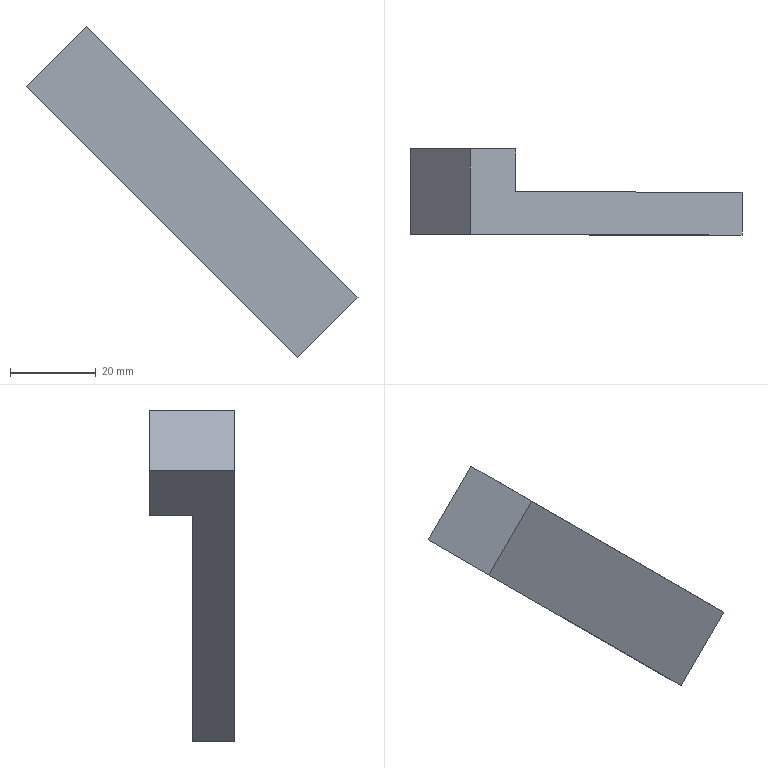Part | NX | features solid 2 | 1 solid | 8 faces | box 77.441 x 20 x 77.441 mm | volume 20790 mm3 | plane 8
STEP:
#1=CARTESIAN_POINT('',(-977.428,40.,-121.263));
#2=VERTEX_POINT('',#1);
#3=CARTESIAN_POINT('',(-963.381,40.,-107.216));
#4=VERTEX_POINT('',#3);
#5=CARTESIAN_POINT('',(-964.397,40.,-108.232));
#6=DIRECTION('',(0.7071,0.,0.7071));
#7=VECTOR('',#6,1000.);
#8=LINE('',#5,#7);
#9=EDGE_CURVE('',#2,#4,#8,.T.);
#10=ORIENTED_EDGE('',*,*,#9,.F.);
#11=CARTESIAN_POINT('',(-1030.215,40.,-68.476));
#12=VERTEX_POINT('',#11);
#13=CARTESIAN_POINT('',(-1036.273,40.,-62.418));
#14=DIRECTION('',(-0.7071,0.,0.7071));
#15=VECTOR('',#14,1000.);
#16=LINE('',#13,#15);
#17=EDGE_CURVE('',#12,#2,#16,.F.);
#18=ORIENTED_EDGE('',*,*,#17,.F.);
#19=CARTESIAN_POINT('',(-1016.168,40.,-54.429));
#20=VERTEX_POINT('',#19);
#21=CARTESIAN_POINT('',(-1017.184,40.,-55.445));
#22=DIRECTION('',(-0.7071,0.,-0.7071));
#23=VECTOR('',#22,1000.);
#24=LINE('',#21,#23);
#25=EDGE_CURVE('',#20,#12,#24,.T.);
#26=ORIENTED_EDGE('',*,*,#25,.F.);
#27=CARTESIAN_POINT('',(-1030.192,40.,-40.405));
#28=DIRECTION('',(0.7071,0.,-0.7071));
#29=VECTOR('',#28,1000.);
#30=LINE('',#27,#29);
#31=EDGE_CURVE('',#20,#4,#30,.T.);
#32=ORIENTED_EDGE('',*,*,#31,.T.);
#33=EDGE_LOOP('',(#10,#18,#26,#32));
#34=FACE_BOUND('',#33,.T.);
#35=CARTESIAN_POINT('',(-1031.207,40.,-41.421));
#36=DIRECTION('',(0.,-1.,0.));
#37=DIRECTION('',(0.9796,0.,0.2008));
#38=AXIS2_PLACEMENT_3D('',#35,#36,#37);
#39=PLANE('',#38);
#40=ADVANCED_FACE('',(#34),#39,.F.);
#41=CARTESIAN_POINT('',(-1030.215,50.,-68.476));
#42=VERTEX_POINT('',#41);
#43=CARTESIAN_POINT('',(-1030.215,40.,-68.476));
#44=DIRECTION('',(0.,1.,0.));
#45=VECTOR('',#44,1000.);
#46=LINE('',#43,#45);
#47=EDGE_CURVE('',#42,#12,#46,.F.);
#48=ORIENTED_EDGE('',*,*,#47,.T.);
#49=ORIENTED_EDGE('',*,*,#17,.T.);
#50=CARTESIAN_POINT('',(-977.428,30.,-121.263));
#51=VERTEX_POINT('',#50);
#52=CARTESIAN_POINT('',(-977.428,40.,-121.263));
#53=DIRECTION('',(0.,-1.,0.));
#54=VECTOR('',#53,1000.);
#55=LINE('',#52,#54);
#56=EDGE_CURVE('',#51,#2,#55,.F.);
#57=ORIENTED_EDGE('',*,*,#56,.F.);
#58=CARTESIAN_POINT('',(-1040.822,30.,-57.869));
#59=VERTEX_POINT('',#58);
#60=CARTESIAN_POINT('',(-1036.273,30.,-62.418));
#61=DIRECTION('',(-0.7071,0.,0.7071));
#62=VECTOR('',#61,1000.);
#63=LINE('',#60,#62);
#64=EDGE_CURVE('',#59,#51,#63,.F.);
#65=ORIENTED_EDGE('',*,*,#64,.F.);
#66=CARTESIAN_POINT('',(-1040.822,50.,-57.869));
#67=VERTEX_POINT('',#66);
#68=CARTESIAN_POINT('',(-1040.822,40.,-57.869));
#69=DIRECTION('',(0.,1.,0.));
#70=VECTOR('',#69,1000.);
#71=LINE('',#68,#70);
#72=EDGE_CURVE('',#67,#59,#71,.F.);
#73=ORIENTED_EDGE('',*,*,#72,.F.);
#74=CARTESIAN_POINT('',(-1036.273,50.,-62.418));
#75=DIRECTION('',(-0.7071,0.,0.7071));
#76=VECTOR('',#75,1000.);
#77=LINE('',#74,#76);
#78=EDGE_CURVE('',#67,#42,#77,.F.);
#79=ORIENTED_EDGE('',*,*,#78,.T.);
#80=EDGE_LOOP('',(#48,#49,#57,#65,#73,#79));
#81=FACE_BOUND('',#80,.T.);
#82=CARTESIAN_POINT('',(-1036.273,40.,-62.418));
#83=DIRECTION('',(-0.7071,0.,-0.7071));
#84=DIRECTION('',(0.7071,0.,-0.7071));
#85=AXIS2_PLACEMENT_3D('',#82,#83,#84);
#86=PLANE('',#85);
#87=ADVANCED_FACE('',(#81),#86,.T.);
#88=CARTESIAN_POINT('',(-963.381,30.,-107.216));
#89=VERTEX_POINT('',#88);
#90=CARTESIAN_POINT('',(-963.381,40.,-107.216));
#91=DIRECTION('',(0.,-1.,0.));
#92=VECTOR('',#91,1000.);
#93=LINE('',#90,#92);
#94=EDGE_CURVE('',#4,#89,#93,.T.);
#95=ORIENTED_EDGE('',*,*,#94,.F.);
#96=ORIENTED_EDGE('',*,*,#31,.F.);
#97=CARTESIAN_POINT('',(-1016.168,50.,-54.429));
#98=VERTEX_POINT('',#97);
#99=CARTESIAN_POINT('',(-1016.168,40.,-54.429));
#100=DIRECTION('',(0.,1.,0.));
#101=VECTOR('',#100,1000.);
#102=LINE('',#99,#101);
#103=EDGE_CURVE('',#20,#98,#102,.T.);
#104=ORIENTED_EDGE('',*,*,#103,.T.);
#105=CARTESIAN_POINT('',(-1026.775,50.,-43.822));
#106=VERTEX_POINT('',#105);
#107=CARTESIAN_POINT('',(-1030.192,50.,-40.405));
#108=DIRECTION('',(0.7071,0.,-0.7071));
#109=VECTOR('',#108,1000.);
#110=LINE('',#107,#109);
#111=EDGE_CURVE('',#106,#98,#110,.T.);
#112=ORIENTED_EDGE('',*,*,#111,.F.);
#113=CARTESIAN_POINT('',(-1026.775,30.,-43.822));
#114=VERTEX_POINT('',#113);
#115=CARTESIAN_POINT('',(-1026.775,40.,-43.822));
#116=DIRECTION('',(0.,1.,0.));
#117=VECTOR('',#116,1000.);
#118=LINE('',#115,#117);
#119=EDGE_CURVE('',#114,#106,#118,.T.);
#120=ORIENTED_EDGE('',*,*,#119,.F.);
#121=CARTESIAN_POINT('',(-1030.192,30.,-40.405));
#122=DIRECTION('',(0.7071,0.,-0.7071));
#123=VECTOR('',#122,1000.);
#124=LINE('',#121,#123);
#125=EDGE_CURVE('',#114,#89,#124,.T.);
#126=ORIENTED_EDGE('',*,*,#125,.T.);
#127=EDGE_LOOP('',(#95,#96,#104,#112,#120,#126));
#128=FACE_BOUND('',#127,.T.);
#129=CARTESIAN_POINT('',(-1023.864,40.,-46.733));
#130=DIRECTION('',(-0.7071,0.,-0.7071));
#131=DIRECTION('',(0.7071,0.,-0.7071));
#132=AXIS2_PLACEMENT_3D('',#129,#130,#131);
#133=PLANE('',#132);
#134=ADVANCED_FACE('',(#128),#133,.F.);
#135=ORIENTED_EDGE('',*,*,#64,.T.);
#136=CARTESIAN_POINT('',(-964.397,30.,-108.232));
#137=DIRECTION('',(0.7071,0.,0.7071));
#138=VECTOR('',#137,1000.);
#139=LINE('',#136,#138);
#140=EDGE_CURVE('',#51,#89,#139,.T.);
#141=ORIENTED_EDGE('',*,*,#140,.T.);
#142=ORIENTED_EDGE('',*,*,#125,.F.);
#143=CARTESIAN_POINT('',(-1027.79,30.,-44.838));
#144=DIRECTION('',(-0.7071,0.,-0.7071));
#145=VECTOR('',#144,1000.);
#146=LINE('',#143,#145);
#147=EDGE_CURVE('',#114,#59,#146,.T.);
#148=ORIENTED_EDGE('',*,*,#147,.T.);
#149=EDGE_LOOP('',(#135,#141,#142,#148));
#150=FACE_BOUND('',#149,.T.);
#151=CARTESIAN_POINT('',(-1031.207,30.,-41.421));
#152=DIRECTION('',(0.,-1.,0.));
#153=DIRECTION('',(0.9796,0.,0.2008));
#154=AXIS2_PLACEMENT_3D('',#151,#152,#153);
#155=PLANE('',#154);
#156=ADVANCED_FACE('',(#150),#155,.T.);
#157=CARTESIAN_POINT('',(-1027.79,50.,-44.838));
#158=DIRECTION('',(-0.7071,0.,-0.7071));
#159=VECTOR('',#158,1000.);
#160=LINE('',#157,#159);
#161=EDGE_CURVE('',#106,#67,#160,.T.);
#162=ORIENTED_EDGE('',*,*,#161,.F.);
#163=ORIENTED_EDGE('',*,*,#111,.T.);
#164=CARTESIAN_POINT('',(-1017.184,50.,-55.445));
#165=DIRECTION('',(-0.7071,0.,-0.7071));
#166=VECTOR('',#165,1000.);
#167=LINE('',#164,#166);
#168=EDGE_CURVE('',#98,#42,#167,.T.);
#169=ORIENTED_EDGE('',*,*,#168,.T.);
#170=ORIENTED_EDGE('',*,*,#78,.F.);
#171=EDGE_LOOP('',(#162,#163,#169,#170));
#172=FACE_BOUND('',#171,.T.);
#173=CARTESIAN_POINT('',(-1031.207,50.,-41.421));
#174=DIRECTION('',(0.,-1.,0.));
#175=DIRECTION('',(0.9796,0.,0.2008));
#176=AXIS2_PLACEMENT_3D('',#173,#174,#175);
#177=PLANE('',#176);
#178=ADVANCED_FACE('',(#172),#177,.F.);
#179=ORIENTED_EDGE('',*,*,#56,.T.);
#180=ORIENTED_EDGE('',*,*,#9,.T.);
#181=ORIENTED_EDGE('',*,*,#94,.T.);
#182=ORIENTED_EDGE('',*,*,#140,.F.);
#183=EDGE_LOOP('',(#179,#180,#181,#182));
#184=FACE_BOUND('',#183,.T.);
#185=CARTESIAN_POINT('',(-993.082,180.,-136.918));
#186=DIRECTION('',(0.7071,0.,-0.7071));
#187=DIRECTION('',(-0.7071,0.,-0.7071));
#188=AXIS2_PLACEMENT_3D('',#185,#186,#187);
#189=PLANE('',#188);
#190=ADVANCED_FACE('',(#184),#189,.T.);
#191=ORIENTED_EDGE('',*,*,#147,.F.);
#192=ORIENTED_EDGE('',*,*,#119,.T.);
#193=ORIENTED_EDGE('',*,*,#161,.T.);
#194=ORIENTED_EDGE('',*,*,#72,.T.);
#195=EDGE_LOOP('',(#191,#192,#193,#194));
#196=FACE_BOUND('',#195,.T.);
#197=CARTESIAN_POINT('',(-1029.012,320.,-46.059));
#198=DIRECTION('',(-0.7071,0.,0.7071));
#199=DIRECTION('',(0.7071,0.,0.7071));
#200=AXIS2_PLACEMENT_3D('',#197,#198,#199);
#201=PLANE('',#200);
#202=ADVANCED_FACE('',(#196),#201,.T.);
#203=ORIENTED_EDGE('',*,*,#103,.F.);
#204=ORIENTED_EDGE('',*,*,#25,.T.);
#205=ORIENTED_EDGE('',*,*,#47,.F.);
#206=ORIENTED_EDGE('',*,*,#168,.F.);
#207=EDGE_LOOP('',(#203,#204,#205,#206));
#208=FACE_BOUND('',#207,.T.);
#209=CARTESIAN_POINT('',(-1018.405,320.,-56.666));
#210=DIRECTION('',(-0.7071,0.,0.7071));
#211=DIRECTION('',(0.7071,0.,0.7071));
#212=AXIS2_PLACEMENT_3D('',#209,#210,#211);
#213=PLANE('',#212);
#214=ADVANCED_FACE('',(#208),#213,.F.);
#215=CLOSED_SHELL('',(#40,#87,#134,#156,#178,#190,#202,#214));
#216=MANIFOLD_SOLID_BREP('',#215);
#217=(LENGTH_UNIT()NAMED_UNIT(*)SI_UNIT(.MILLI.,.METRE.));
#218=UNCERTAINTY_MEASURE_WITH_UNIT(LENGTH_MEASURE(0.00001),#217,'','');
#219=(NAMED_UNIT(*)PLANE_ANGLE_UNIT()SI_UNIT($,.RADIAN.));
#220=(NAMED_UNIT(*)SI_UNIT($,.STERADIAN.)SOLID_ANGLE_UNIT());
#221=(GEOMETRIC_REPRESENTATION_CONTEXT(3)GLOBAL_UNCERTAINTY_ASSIGNED_CONTEXT((#218))GLOBAL_UNIT_ASSIGNED_CONTEXT((#217,#219,#220))REPRESENTATION_CONTEXT('',''));
#222=ADVANCED_BREP_SHAPE_REPRESENTATION('',(#216),#221);